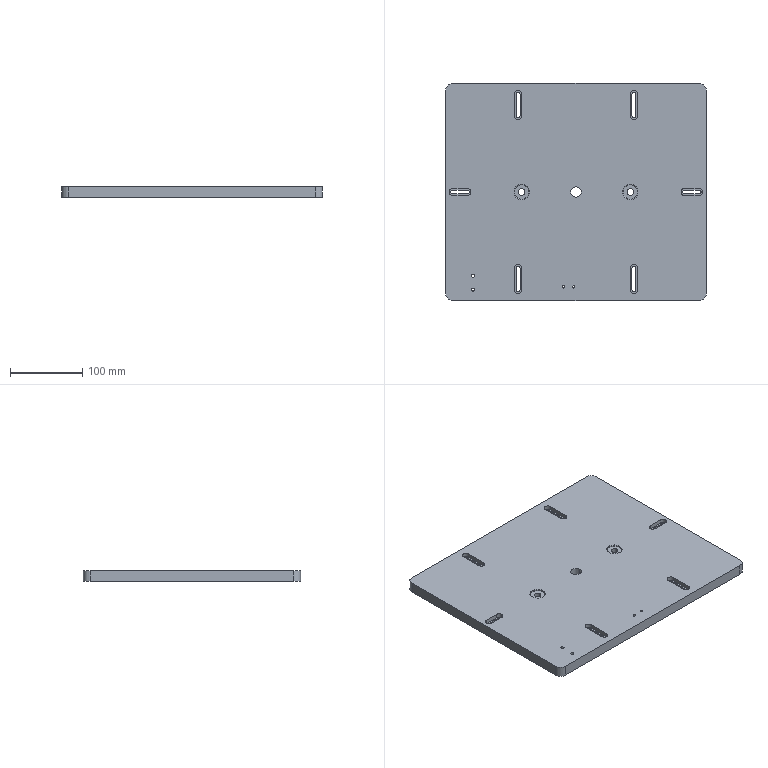Part | STEP file | KF-2212-050-004 | 1 solid | 96 faces | box 360 x 300 x 15 mm | volume 1590631 mm3 | cylinder 50 | plane 38 | cone 8 | commonest cylinder face diameters 5.5 x14 10 x14 20 x8 3.3 x4 4.2 x4 9 x4